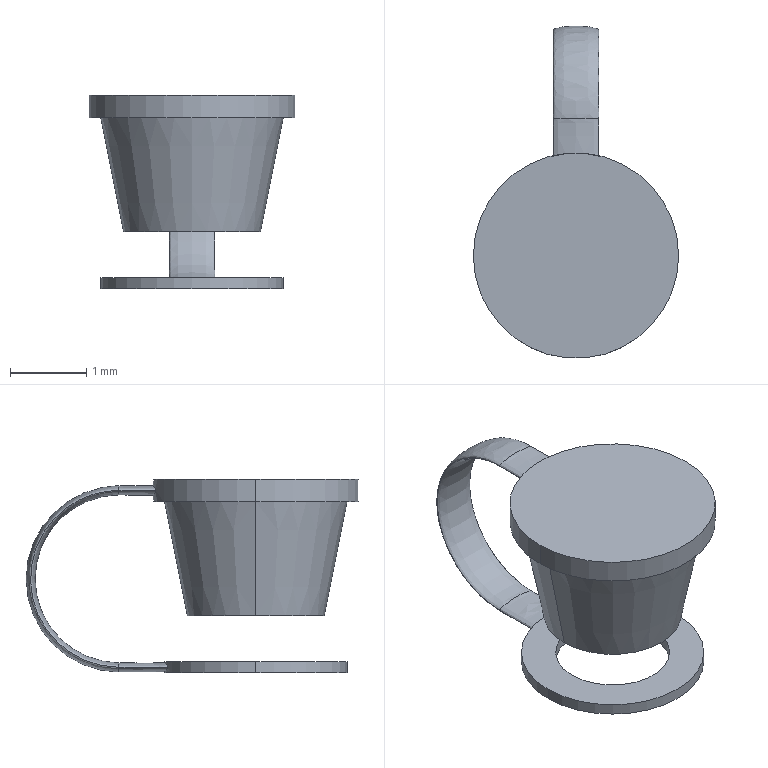Part | STEP file | 2026.6.15-Main Assembly图.sldasm-Part-226 | 1 solid | 24 faces | box 2.7 x 4.372 x 2.55 mm | volume 4.734 mm3 | cylinder 8 | plane 7 | spline 7 | cone 2 | commonest cylinder face diameters 1.5 x4 2.4 x2 2.7 x2